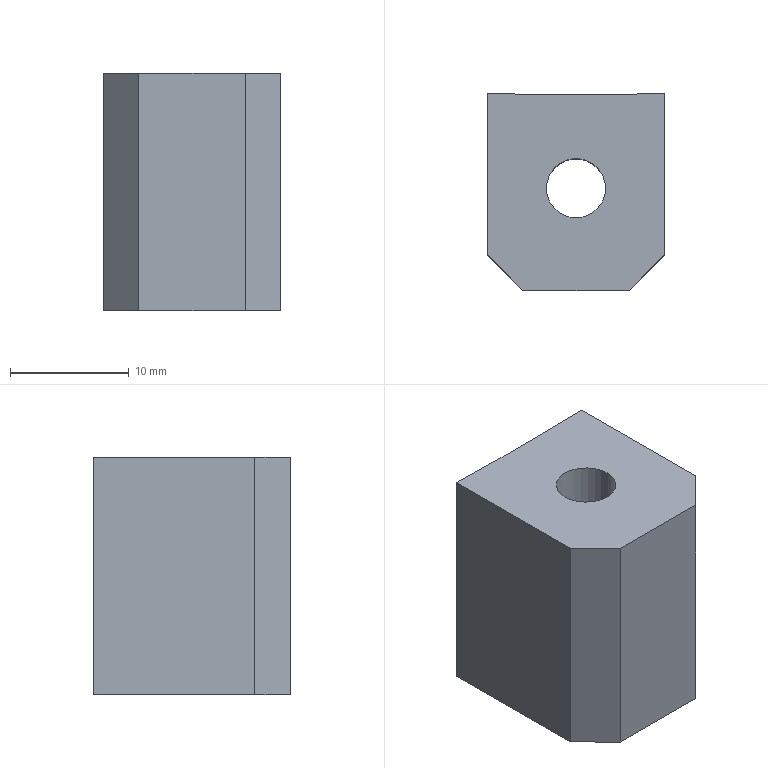Part | SolidWorks | features Chamfer 1, Extrusion 1, HoleWzd 1 | 1 solid | 10 faces | box 15 x 16.6 x 20 mm | volume 4383 mm3 | plane 7 | cylinder 3 | commonest cylinder face diameters 5 x2 462.6 x1
STEP:
#1=CARTESIAN_POINT('',(-2.5,-239.178,0.));
#2=VERTEX_POINT('',#1);
#3=CARTESIAN_POINT('',(2.5,-239.178,0.));
#4=VERTEX_POINT('',#3);
#5=CARTESIAN_POINT('',(0.,-239.178,0.));
#6=DIRECTION('',(0.,0.,1.));
#7=DIRECTION('',(1.,0.,0.));
#8=AXIS2_PLACEMENT_3D('',#5,#6,#7);
#9=CIRCLE('',#8,2.5);
#10=EDGE_CURVE('',#2,#4,#9,.T.);
#11=ORIENTED_EDGE('',*,*,#10,.F.);
#12=CARTESIAN_POINT('',(-2.5,-239.178,20.));
#13=VERTEX_POINT('',#12);
#14=CARTESIAN_POINT('',(-2.5,-239.178,20.));
#15=DIRECTION('',(0.,0.,1.));
#16=VECTOR('',#15,1000.);
#17=LINE('',#14,#16);
#18=EDGE_CURVE('',#2,#13,#17,.T.);
#19=ORIENTED_EDGE('',*,*,#18,.T.);
#20=CARTESIAN_POINT('',(2.5,-239.178,20.));
#21=VERTEX_POINT('',#20);
#22=CARTESIAN_POINT('',(0.,-239.178,20.));
#23=DIRECTION('',(0.,0.,1.));
#24=DIRECTION('',(1.,0.,0.));
#25=AXIS2_PLACEMENT_3D('',#22,#23,#24);
#26=CIRCLE('',#25,2.5);
#27=EDGE_CURVE('',#13,#21,#26,.T.);
#28=ORIENTED_EDGE('',*,*,#27,.T.);
#29=CARTESIAN_POINT('',(2.5,-239.178,20.));
#30=DIRECTION('',(0.,0.,1.));
#31=VECTOR('',#30,1000.);
#32=LINE('',#29,#31);
#33=EDGE_CURVE('',#4,#21,#32,.T.);
#34=ORIENTED_EDGE('',*,*,#33,.F.);
#35=EDGE_LOOP('',(#11,#19,#28,#34));
#36=FACE_OUTER_BOUND('',#35,.T.);
#37=CARTESIAN_POINT('',(0.,-239.178,20.));
#38=DIRECTION('',(0.,0.,1.));
#39=DIRECTION('',(1.,0.,0.));
#40=AXIS2_PLACEMENT_3D('',#37,#38,#39);
#41=CYLINDRICAL_SURFACE('',#40,2.5);
#42=ADVANCED_FACE('',(#36),#41,.F.);
#43=CARTESIAN_POINT('',(7.5,-231.178,0.));
#44=VERTEX_POINT('',#43);
#45=CARTESIAN_POINT('',(-7.5,-231.178,0.));
#46=VERTEX_POINT('',#45);
#47=CARTESIAN_POINT('',(0.,0.,0.));
#48=DIRECTION('',(0.,0.,-1.));
#49=DIRECTION('',(1.,0.,0.));
#50=AXIS2_PLACEMENT_3D('',#47,#48,#49);
#51=CIRCLE('',#50,231.3);
#52=EDGE_CURVE('',#44,#46,#51,.T.);
#53=ORIENTED_EDGE('',*,*,#52,.T.);
#54=CARTESIAN_POINT('',(-7.5,-231.178,20.));
#55=VERTEX_POINT('',#54);
#56=CARTESIAN_POINT('',(-7.5,-231.178,20.));
#57=DIRECTION('',(0.,0.,-1.));
#58=VECTOR('',#57,1000.);
#59=LINE('',#56,#58);
#60=EDGE_CURVE('',#55,#46,#59,.T.);
#61=ORIENTED_EDGE('',*,*,#60,.F.);
#62=CARTESIAN_POINT('',(7.5,-231.178,20.));
#63=VERTEX_POINT('',#62);
#64=CARTESIAN_POINT('',(0.,0.,20.));
#65=DIRECTION('',(0.,0.,-1.));
#66=DIRECTION('',(1.,0.,0.));
#67=AXIS2_PLACEMENT_3D('',#64,#65,#66);
#68=CIRCLE('',#67,231.3);
#69=EDGE_CURVE('',#63,#55,#68,.T.);
#70=ORIENTED_EDGE('',*,*,#69,.F.);
#71=CARTESIAN_POINT('',(7.5,-231.178,20.));
#72=DIRECTION('',(0.,0.,-1.));
#73=VECTOR('',#72,1000.);
#74=LINE('',#71,#73);
#75=EDGE_CURVE('',#63,#44,#74,.T.);
#76=ORIENTED_EDGE('',*,*,#75,.T.);
#77=EDGE_LOOP('',(#53,#61,#70,#76));
#78=FACE_OUTER_BOUND('',#77,.T.);
#79=CARTESIAN_POINT('',(0.,0.,20.));
#80=DIRECTION('',(0.,0.,-1.));
#81=DIRECTION('',(-1.,0.,0.));
#82=AXIS2_PLACEMENT_3D('',#79,#80,#81);
#83=CYLINDRICAL_SURFACE('',#82,231.3);
#84=ADVANCED_FACE('',(#78),#83,.F.);
#85=CARTESIAN_POINT('',(-7.5,-244.778,0.));
#86=VERTEX_POINT('',#85);
#87=CARTESIAN_POINT('',(-7.5,-231.178,0.));
#88=DIRECTION('',(0.,-1.,0.));
#89=VECTOR('',#88,1000.);
#90=LINE('',#87,#89);
#91=EDGE_CURVE('',#46,#86,#90,.T.);
#92=ORIENTED_EDGE('',*,*,#91,.T.);
#93=CARTESIAN_POINT('',(-7.5,-244.778,20.));
#94=VERTEX_POINT('',#93);
#95=CARTESIAN_POINT('',(-7.5,-244.778,20.));
#96=DIRECTION('',(0.,0.,1.));
#97=VECTOR('',#96,1000.);
#98=LINE('',#95,#97);
#99=EDGE_CURVE('',#86,#94,#98,.T.);
#100=ORIENTED_EDGE('',*,*,#99,.T.);
#101=CARTESIAN_POINT('',(-7.5,-231.178,20.));
#102=DIRECTION('',(0.,-1.,0.));
#103=VECTOR('',#102,1000.);
#104=LINE('',#101,#103);
#105=EDGE_CURVE('',#55,#94,#104,.T.);
#106=ORIENTED_EDGE('',*,*,#105,.F.);
#107=ORIENTED_EDGE('',*,*,#60,.T.);
#108=EDGE_LOOP('',(#92,#100,#106,#107));
#109=FACE_OUTER_BOUND('',#108,.T.);
#110=CARTESIAN_POINT('',(-7.5,-231.178,20.));
#111=DIRECTION('',(1.,0.,0.));
#112=DIRECTION('',(0.,1.,0.));
#113=AXIS2_PLACEMENT_3D('',#110,#111,#112);
#114=PLANE('',#113);
#115=ADVANCED_FACE('',(#109),#114,.F.);
#116=CARTESIAN_POINT('',(-4.5,-247.778,0.));
#117=VERTEX_POINT('',#116);
#118=CARTESIAN_POINT('',(4.5,-247.778,0.));
#119=VERTEX_POINT('',#118);
#120=CARTESIAN_POINT('',(-7.5,-247.778,0.));
#121=DIRECTION('',(1.,0.,0.));
#122=VECTOR('',#121,1000.);
#123=LINE('',#120,#122);
#124=EDGE_CURVE('',#117,#119,#123,.T.);
#125=ORIENTED_EDGE('',*,*,#124,.T.);
#126=CARTESIAN_POINT('',(4.5,-247.778,20.));
#127=VERTEX_POINT('',#126);
#128=CARTESIAN_POINT('',(4.5,-247.778,20.));
#129=DIRECTION('',(0.,0.,1.));
#130=VECTOR('',#129,1000.);
#131=LINE('',#128,#130);
#132=EDGE_CURVE('',#119,#127,#131,.T.);
#133=ORIENTED_EDGE('',*,*,#132,.T.);
#134=CARTESIAN_POINT('',(-4.5,-247.778,20.));
#135=VERTEX_POINT('',#134);
#136=CARTESIAN_POINT('',(-7.5,-247.778,20.));
#137=DIRECTION('',(1.,0.,0.));
#138=VECTOR('',#137,1000.);
#139=LINE('',#136,#138);
#140=EDGE_CURVE('',#135,#127,#139,.T.);
#141=ORIENTED_EDGE('',*,*,#140,.F.);
#142=CARTESIAN_POINT('',(-4.5,-247.778,20.));
#143=DIRECTION('',(0.,0.,-1.));
#144=VECTOR('',#143,1000.);
#145=LINE('',#142,#144);
#146=EDGE_CURVE('',#135,#117,#145,.T.);
#147=ORIENTED_EDGE('',*,*,#146,.T.);
#148=EDGE_LOOP('',(#125,#133,#141,#147));
#149=FACE_OUTER_BOUND('',#148,.T.);
#150=CARTESIAN_POINT('',(-7.5,-247.778,20.));
#151=DIRECTION('',(0.,1.,0.));
#152=DIRECTION('',(0.,0.,1.));
#153=AXIS2_PLACEMENT_3D('',#150,#151,#152);
#154=PLANE('',#153);
#155=ADVANCED_FACE('',(#149),#154,.F.);
#156=CARTESIAN_POINT('',(7.5,-244.778,20.));
#157=VERTEX_POINT('',#156);
#158=CARTESIAN_POINT('',(7.5,-247.778,20.));
#159=DIRECTION('',(0.,1.,0.));
#160=VECTOR('',#159,1000.);
#161=LINE('',#158,#160);
#162=EDGE_CURVE('',#157,#63,#161,.T.);
#163=ORIENTED_EDGE('',*,*,#162,.F.);
#164=CARTESIAN_POINT('',(7.5,-244.778,0.));
#165=VERTEX_POINT('',#164);
#166=CARTESIAN_POINT('',(7.5,-244.778,20.));
#167=DIRECTION('',(0.,0.,-1.));
#168=VECTOR('',#167,1000.);
#169=LINE('',#166,#168);
#170=EDGE_CURVE('',#157,#165,#169,.T.);
#171=ORIENTED_EDGE('',*,*,#170,.T.);
#172=CARTESIAN_POINT('',(7.5,-247.778,0.));
#173=DIRECTION('',(0.,1.,0.));
#174=VECTOR('',#173,1000.);
#175=LINE('',#172,#174);
#176=EDGE_CURVE('',#165,#44,#175,.T.);
#177=ORIENTED_EDGE('',*,*,#176,.T.);
#178=ORIENTED_EDGE('',*,*,#75,.F.);
#179=EDGE_LOOP('',(#163,#171,#177,#178));
#180=FACE_OUTER_BOUND('',#179,.T.);
#181=CARTESIAN_POINT('',(7.5,-247.778,20.));
#182=DIRECTION('',(-1.,0.,0.));
#183=DIRECTION('',(0.,-1.,0.));
#184=AXIS2_PLACEMENT_3D('',#181,#182,#183);
#185=PLANE('',#184);
#186=ADVANCED_FACE('',(#180),#185,.F.);
#187=CARTESIAN_POINT('',(0.,-239.178,20.));
#188=DIRECTION('',(0.,0.,1.));
#189=DIRECTION('',(1.,0.,0.));
#190=AXIS2_PLACEMENT_3D('',#187,#188,#189);
#191=CIRCLE('',#190,2.5);
#192=EDGE_CURVE('',#21,#13,#191,.T.);
#193=ORIENTED_EDGE('',*,*,#192,.F.);
#194=ORIENTED_EDGE('',*,*,#27,.F.);
#195=EDGE_LOOP('',(#193,#194));
#196=FACE_BOUND('',#195,.T.);
#197=ORIENTED_EDGE('',*,*,#140,.T.);
#198=CARTESIAN_POINT('',(126.139,-126.139,20.));
#199=DIRECTION('',(0.7071,0.7071,0.));
#200=VECTOR('',#199,1000.);
#201=LINE('',#198,#200);
#202=EDGE_CURVE('',#127,#157,#201,.T.);
#203=ORIENTED_EDGE('',*,*,#202,.T.);
#204=ORIENTED_EDGE('',*,*,#162,.T.);
#205=ORIENTED_EDGE('',*,*,#69,.T.);
#206=ORIENTED_EDGE('',*,*,#105,.T.);
#207=CARTESIAN_POINT('',(-126.139,-126.139,20.));
#208=DIRECTION('',(0.7071,-0.7071,0.));
#209=VECTOR('',#208,1000.);
#210=LINE('',#207,#209);
#211=EDGE_CURVE('',#94,#135,#210,.T.);
#212=ORIENTED_EDGE('',*,*,#211,.T.);
#213=EDGE_LOOP('',(#197,#203,#204,#205,#206,#212));
#214=FACE_OUTER_BOUND('',#213,.T.);
#215=CARTESIAN_POINT('',(0.,0.,20.));
#216=DIRECTION('',(0.,0.,1.));
#217=DIRECTION('',(1.,0.,0.));
#218=AXIS2_PLACEMENT_3D('',#215,#216,#217);
#219=PLANE('',#218);
#220=ADVANCED_FACE('',(#196,#214),#219,.T.);
#221=CARTESIAN_POINT('',(0.,-239.178,0.));
#222=DIRECTION('',(0.,0.,1.));
#223=DIRECTION('',(1.,0.,0.));
#224=AXIS2_PLACEMENT_3D('',#221,#222,#223);
#225=CIRCLE('',#224,2.5);
#226=EDGE_CURVE('',#4,#2,#225,.T.);
#227=ORIENTED_EDGE('',*,*,#226,.T.);
#228=ORIENTED_EDGE('',*,*,#10,.T.);
#229=EDGE_LOOP('',(#227,#228));
#230=FACE_BOUND('',#229,.T.);
#231=ORIENTED_EDGE('',*,*,#176,.F.);
#232=CARTESIAN_POINT('',(7.5,-244.778,0.));
#233=DIRECTION('',(-0.7071,-0.7071,0.));
#234=VECTOR('',#233,1000.);
#235=LINE('',#232,#234);
#236=EDGE_CURVE('',#165,#119,#235,.T.);
#237=ORIENTED_EDGE('',*,*,#236,.T.);
#238=ORIENTED_EDGE('',*,*,#124,.F.);
#239=CARTESIAN_POINT('',(-4.5,-247.778,0.));
#240=DIRECTION('',(-0.7071,0.7071,0.));
#241=VECTOR('',#240,1000.);
#242=LINE('',#239,#241);
#243=EDGE_CURVE('',#117,#86,#242,.T.);
#244=ORIENTED_EDGE('',*,*,#243,.T.);
#245=ORIENTED_EDGE('',*,*,#91,.F.);
#246=ORIENTED_EDGE('',*,*,#52,.F.);
#247=EDGE_LOOP('',(#231,#237,#238,#244,#245,#246));
#248=FACE_OUTER_BOUND('',#247,.T.);
#249=CARTESIAN_POINT('',(0.,0.,0.));
#250=DIRECTION('',(0.,0.,1.));
#251=DIRECTION('',(1.,0.,0.));
#252=AXIS2_PLACEMENT_3D('',#249,#250,#251);
#253=PLANE('',#252);
#254=ADVANCED_FACE('',(#230,#248),#253,.F.);
#255=ORIENTED_EDGE('',*,*,#202,.F.);
#256=ORIENTED_EDGE('',*,*,#132,.F.);
#257=ORIENTED_EDGE('',*,*,#236,.F.);
#258=ORIENTED_EDGE('',*,*,#170,.F.);
#259=EDGE_LOOP('',(#255,#256,#257,#258));
#260=FACE_OUTER_BOUND('',#259,.T.);
#261=CARTESIAN_POINT('',(7.5,-244.778,20.));
#262=DIRECTION('',(-0.7071,0.7071,0.));
#263=DIRECTION('',(0.,0.,-1.));
#264=AXIS2_PLACEMENT_3D('',#261,#262,#263);
#265=PLANE('',#264);
#266=ADVANCED_FACE('',(#260),#265,.F.);
#267=ORIENTED_EDGE('',*,*,#211,.F.);
#268=ORIENTED_EDGE('',*,*,#99,.F.);
#269=ORIENTED_EDGE('',*,*,#243,.F.);
#270=ORIENTED_EDGE('',*,*,#146,.F.);
#271=EDGE_LOOP('',(#267,#268,#269,#270));
#272=FACE_OUTER_BOUND('',#271,.T.);
#273=CARTESIAN_POINT('',(-4.5,-247.778,20.));
#274=DIRECTION('',(0.7071,0.7071,0.));
#275=DIRECTION('',(0.,0.,-1.));
#276=AXIS2_PLACEMENT_3D('',#273,#274,#275);
#277=PLANE('',#276);
#278=ADVANCED_FACE('',(#272),#277,.F.);
#279=ORIENTED_EDGE('',*,*,#18,.F.);
#280=ORIENTED_EDGE('',*,*,#226,.F.);
#281=ORIENTED_EDGE('',*,*,#33,.T.);
#282=ORIENTED_EDGE('',*,*,#192,.T.);
#283=EDGE_LOOP('',(#279,#280,#281,#282));
#284=FACE_OUTER_BOUND('',#283,.T.);
#285=CARTESIAN_POINT('',(0.,-239.178,20.));
#286=DIRECTION('',(0.,0.,1.));
#287=DIRECTION('',(1.,0.,0.));
#288=AXIS2_PLACEMENT_3D('',#285,#286,#287);
#289=CYLINDRICAL_SURFACE('',#288,2.5);
#290=ADVANCED_FACE('',(#284),#289,.F.);
#291=CLOSED_SHELL('',(#42,#84,#115,#155,#186,#220,#254,#266,#278,#290));
#292=MANIFOLD_SOLID_BREP('',#291);
#293=CARTESIAN_POINT('',(0.,0.,0.));
#294=DIRECTION('',(0.,0.,1.));
#295=DIRECTION('',(1.,0.,0.));
#296=AXIS2_PLACEMENT_3D('',#293,#294,#295);
#297=(LENGTH_UNIT()NAMED_UNIT(*)SI_UNIT(.MILLI.,.METRE.));
#298=UNCERTAINTY_MEASURE_WITH_UNIT(LENGTH_MEASURE(0.00001),#297,'','');
#299=(NAMED_UNIT(*)PLANE_ANGLE_UNIT()SI_UNIT($,.RADIAN.));
#300=(NAMED_UNIT(*)SI_UNIT($,.STERADIAN.)SOLID_ANGLE_UNIT());
#301=(GEOMETRIC_REPRESENTATION_CONTEXT(3)GLOBAL_UNCERTAINTY_ASSIGNED_CONTEXT((#298))GLOBAL_UNIT_ASSIGNED_CONTEXT((#297,#299,#300))REPRESENTATION_CONTEXT('',''));
#302=ADVANCED_BREP_SHAPE_REPRESENTATION('',(#292,#296),#301);